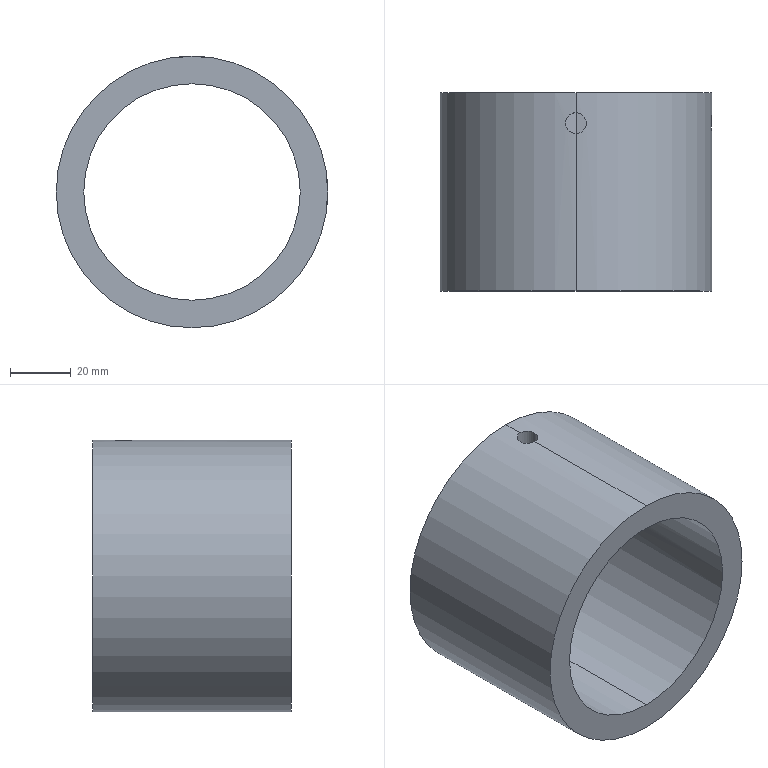Part | SolidWorks | features ICE 2, 3DProfileFeature 1, Extrusion 1, HoleWzd 1 | 1 solid | 10 faces | box 89 x 65 x 89 mm | volume 146372 mm3 | cylinder 8 | plane 2 | commonest cylinder face diameters 6.8 x4 71 x2 89 x2
STEP:
#1=CARTESIAN_POINT('',(0.,51.6,35.5));
#2=VERTEX_POINT('',#1);
#3=CARTESIAN_POINT('',(-3.4,55.,35.337));
#4=VERTEX_POINT('',#3);
#5=CARTESIAN_POINT('',(0.,51.6,35.5));
#6=CARTESIAN_POINT('',(-0.2219,51.6,35.5));
#7=CARTESIAN_POINT('',(-0.4472,51.622,35.498));
#8=CARTESIAN_POINT('',(-0.8832,51.709,35.49));
#9=CARTESIAN_POINT('',(-1.095,51.774,35.484));
#10=CARTESIAN_POINT('',(-1.507,51.944,35.469));
#11=CARTESIAN_POINT('',(-1.706,52.051,35.459));
#12=CARTESIAN_POINT('',(-2.074,52.297,35.44));
#13=CARTESIAN_POINT('',(-2.246,52.437,35.429));
#14=CARTESIAN_POINT('',(-2.563,52.755,35.408));
#15=CARTESIAN_POINT('',(-2.703,52.926,35.397));
#16=CARTESIAN_POINT('',(-2.95,53.294,35.377));
#17=CARTESIAN_POINT('',(-3.056,53.493,35.368));
#18=CARTESIAN_POINT('',(-3.227,53.905,35.353));
#19=CARTESIAN_POINT('',(-3.291,54.117,35.347));
#20=CARTESIAN_POINT('',(-3.378,54.553,35.339));
#21=CARTESIAN_POINT('',(-3.4,54.778,35.337));
#22=CARTESIAN_POINT('',(-3.4,55.,35.337));
#23=B_SPLINE_CURVE_WITH_KNOTS('',3,(#5,#6,#7,#8,#9,#10,#11,#12,#13,#14,#15,#16,#17,#18,#19,#20,#21,#22),.UNSPECIFIED.,.F.,.F.,(4,2,2,2,2,2,2,2,4),(0.005319,0.005984,0.006648,0.007313,0.007978,0.008642,0.009307,0.009971,0.01064),.UNSPECIFIED.);
#24=EDGE_CURVE('',#2,#4,#23,.T.);
#25=ORIENTED_EDGE('',*,*,#24,.T.);
#26=CARTESIAN_POINT('',(-3.4,55.,44.37));
#27=VERTEX_POINT('',#26);
#28=CARTESIAN_POINT('',(-3.4,55.,34.5));
#29=DIRECTION('',(0.,0.,1.));
#30=VECTOR('',#29,1000.);
#31=LINE('',#28,#30);
#32=EDGE_CURVE('',#4,#27,#31,.T.);
#33=ORIENTED_EDGE('',*,*,#32,.T.);
#34=CARTESIAN_POINT('',(0.,51.6,44.5));
#35=VERTEX_POINT('',#34);
#36=CARTESIAN_POINT('',(0.,51.6,44.5));
#37=CARTESIAN_POINT('',(-0.2218,51.6,44.5));
#38=CARTESIAN_POINT('',(-0.4471,51.622,44.498));
#39=CARTESIAN_POINT('',(-0.8831,51.709,44.492));
#40=CARTESIAN_POINT('',(-1.095,51.773,44.487));
#41=CARTESIAN_POINT('',(-1.507,51.944,44.475));
#42=CARTESIAN_POINT('',(-1.706,52.05,44.468));
#43=CARTESIAN_POINT('',(-2.074,52.297,44.452));
#44=CARTESIAN_POINT('',(-2.245,52.437,44.444));
#45=CARTESIAN_POINT('',(-2.563,52.755,44.426));
#46=CARTESIAN_POINT('',(-2.703,52.926,44.418));
#47=CARTESIAN_POINT('',(-2.95,53.294,44.402));
#48=CARTESIAN_POINT('',(-3.056,53.493,44.395));
#49=CARTESIAN_POINT('',(-3.227,53.905,44.383));
#50=CARTESIAN_POINT('',(-3.291,54.117,44.378));
#51=CARTESIAN_POINT('',(-3.378,54.553,44.372));
#52=CARTESIAN_POINT('',(-3.4,54.778,44.37));
#53=CARTESIAN_POINT('',(-3.4,55.,44.37));
#54=B_SPLINE_CURVE_WITH_KNOTS('',3,(#36,#37,#38,#39,#40,#41,#42,#43,#44,#45,#46,#47,#48,#49,#50,#51,#52,#53),.UNSPECIFIED.,.F.,.F.,(4,2,2,2,2,2,2,2,4),(0.005318,0.005983,0.006647,0.007312,0.007976,0.00864,0.009305,0.009969,0.01063),.UNSPECIFIED.);
#55=EDGE_CURVE('',#35,#27,#54,.T.);
#56=ORIENTED_EDGE('',*,*,#55,.F.);
#57=CARTESIAN_POINT('',(3.4,55.,44.37));
#58=VERTEX_POINT('',#57);
#59=CARTESIAN_POINT('',(3.4,55.,44.37));
#60=CARTESIAN_POINT('',(3.4,54.775,44.37));
#61=CARTESIAN_POINT('',(3.378,54.554,44.372));
#62=CARTESIAN_POINT('',(3.291,54.119,44.378));
#63=CARTESIAN_POINT('',(3.226,53.903,44.383));
#64=CARTESIAN_POINT('',(3.055,53.492,44.395));
#65=CARTESIAN_POINT('',(2.951,53.296,44.402));
#66=CARTESIAN_POINT('',(2.704,52.927,44.418));
#67=CARTESIAN_POINT('',(2.56,52.752,44.427));
#68=CARTESIAN_POINT('',(2.246,52.438,44.444));
#69=CARTESIAN_POINT('',(2.075,52.297,44.452));
#70=CARTESIAN_POINT('',(1.703,52.049,44.468));
#71=CARTESIAN_POINT('',(1.505,51.943,44.475));
#72=CARTESIAN_POINT('',(1.096,51.774,44.487));
#73=CARTESIAN_POINT('',(0.8817,51.709,44.492));
#74=CARTESIAN_POINT('',(0.4426,51.622,44.498));
#75=CARTESIAN_POINT('',(0.2219,51.6,44.5));
#76=CARTESIAN_POINT('',(0.,51.6,44.5));
#77=B_SPLINE_CURVE_WITH_KNOTS('',3,(#59,#60,#61,#62,#63,#64,#65,#66,#67,#68,#69,#70,#71,#72,#73,#74,#75,#76),.UNSPECIFIED.,.F.,.F.,(4,2,2,2,2,2,2,2,4),(0.,0.0006648,0.00133,0.001994,0.002659,0.003324,0.003989,0.004653,0.005318),.UNSPECIFIED.);
#78=EDGE_CURVE('',#58,#35,#77,.T.);
#79=ORIENTED_EDGE('',*,*,#78,.F.);
#80=CARTESIAN_POINT('',(3.4,55.,35.337));
#81=VERTEX_POINT('',#80);
#82=CARTESIAN_POINT('',(3.4,55.,34.5));
#83=DIRECTION('',(0.,0.,1.));
#84=VECTOR('',#83,1000.);
#85=LINE('',#82,#84);
#86=EDGE_CURVE('',#81,#58,#85,.T.);
#87=ORIENTED_EDGE('',*,*,#86,.F.);
#88=CARTESIAN_POINT('',(3.4,55.,35.337));
#89=CARTESIAN_POINT('',(3.4,54.775,35.337));
#90=CARTESIAN_POINT('',(3.378,54.554,35.339));
#91=CARTESIAN_POINT('',(3.291,54.119,35.347));
#92=CARTESIAN_POINT('',(3.226,53.903,35.353));
#93=CARTESIAN_POINT('',(3.055,53.491,35.368));
#94=CARTESIAN_POINT('',(2.951,53.296,35.377));
#95=CARTESIAN_POINT('',(2.704,52.927,35.397));
#96=CARTESIAN_POINT('',(2.56,52.752,35.408));
#97=CARTESIAN_POINT('',(2.246,52.438,35.429));
#98=CARTESIAN_POINT('',(2.075,52.298,35.44));
#99=CARTESIAN_POINT('',(1.703,52.049,35.46));
#100=CARTESIAN_POINT('',(1.506,51.943,35.469));
#101=CARTESIAN_POINT('',(1.096,51.774,35.484));
#102=CARTESIAN_POINT('',(0.8818,51.709,35.49));
#103=CARTESIAN_POINT('',(0.4427,51.622,35.498));
#104=CARTESIAN_POINT('',(0.222,51.6,35.5));
#105=CARTESIAN_POINT('',(0.,51.6,35.5));
#106=B_SPLINE_CURVE_WITH_KNOTS('',3,(#88,#89,#90,#91,#92,#93,#94,#95,#96,#97,#98,#99,#100,#101,#102,#103,#104,#105),.UNSPECIFIED.,.F.,.F.,(4,2,2,2,2,2,2,2,4),(0.,0.0006649,0.00133,0.001995,0.00266,0.003325,0.003989,0.004654,0.005319),.UNSPECIFIED.);
#107=EDGE_CURVE('',#81,#2,#106,.T.);
#108=ORIENTED_EDGE('',*,*,#107,.T.);
#109=EDGE_LOOP('',(#25,#33,#56,#79,#87,#108));
#110=FACE_OUTER_BOUND('',#109,.T.);
#111=CARTESIAN_POINT('',(0.,55.,34.5));
#112=DIRECTION('',(0.,0.,1.));
#113=DIRECTION('',(1.,0.,0.));
#114=AXIS2_PLACEMENT_3D('',#111,#112,#113);
#115=CYLINDRICAL_SURFACE('',#114,3.4);
#116=ADVANCED_FACE('',(#110),#115,.F.);
#117=CARTESIAN_POINT('',(35.337,55.,-3.4));
#118=VERTEX_POINT('',#117);
#119=CARTESIAN_POINT('',(35.337,55.,3.4));
#120=VERTEX_POINT('',#119);
#121=CARTESIAN_POINT('',(35.337,55.,-3.4));
#122=CARTESIAN_POINT('',(35.337,54.775,-3.4));
#123=CARTESIAN_POINT('',(35.339,54.554,-3.378));
#124=CARTESIAN_POINT('',(35.347,54.119,-3.291));
#125=CARTESIAN_POINT('',(35.353,53.903,-3.226));
#126=CARTESIAN_POINT('',(35.368,53.492,-3.055));
#127=CARTESIAN_POINT('',(35.377,53.296,-2.951));
#128=CARTESIAN_POINT('',(35.397,52.927,-2.704));
#129=CARTESIAN_POINT('',(35.408,52.752,-2.56));
#130=CARTESIAN_POINT('',(35.429,52.439,-2.247));
#131=CARTESIAN_POINT('',(35.44,52.298,-2.076));
#132=CARTESIAN_POINT('',(35.46,52.049,-1.704));
#133=CARTESIAN_POINT('',(35.469,51.944,-1.506));
#134=CARTESIAN_POINT('',(35.484,51.774,-1.097));
#135=CARTESIAN_POINT('',(35.49,51.709,-0.8828));
#136=CARTESIAN_POINT('',(35.498,51.622,-0.4438));
#137=CARTESIAN_POINT('',(35.5,51.6,-0.2231));
#138=CARTESIAN_POINT('',(35.5,51.6,0.2207));
#139=CARTESIAN_POINT('',(35.498,51.622,0.4461));
#140=CARTESIAN_POINT('',(35.49,51.709,0.8823));
#141=CARTESIAN_POINT('',(35.484,51.773,1.094));
#142=CARTESIAN_POINT('',(35.469,51.944,1.506));
#143=CARTESIAN_POINT('',(35.46,52.05,1.705));
#144=CARTESIAN_POINT('',(35.44,52.296,2.073));
#145=CARTESIAN_POINT('',(35.429,52.437,2.245));
#146=CARTESIAN_POINT('',(35.408,52.754,2.563));
#147=CARTESIAN_POINT('',(35.397,52.926,2.703));
#148=CARTESIAN_POINT('',(35.377,53.294,2.949));
#149=CARTESIAN_POINT('',(35.368,53.493,3.056));
#150=CARTESIAN_POINT('',(35.353,53.905,3.226));
#151=CARTESIAN_POINT('',(35.347,54.117,3.291));
#152=CARTESIAN_POINT('',(35.339,54.553,3.378));
#153=CARTESIAN_POINT('',(35.337,54.778,3.4));
#154=CARTESIAN_POINT('',(35.337,55.,3.4));
#155=B_SPLINE_CURVE_WITH_KNOTS('',3,(#121,#122,#123,#124,#125,#126,#127,#128,#129,#130,#131,#132,#133,#134,#135,#136,#137,#138,#139,#140,#141,#142,#143,#144,#145,#146,#147,#148,#149,#150,#151,#152,#153,#154),.UNSPECIFIED.,.F.,.F.,(4,2,2,2,2,2,2,2,2,2,2,2,2,2,2,2,4),(0.,0.0006648,0.00133,0.001994,0.002659,0.003324,0.003989,0.004653,0.005318,0.005983,0.006648,0.007312,0.007977,0.008642,0.009307,0.009971,0.01064),.UNSPECIFIED.);
#156=EDGE_CURVE('',#118,#120,#155,.T.);
#157=ORIENTED_EDGE('',*,*,#156,.T.);
#158=CARTESIAN_POINT('',(44.37,55.,3.4));
#159=VERTEX_POINT('',#158);
#160=CARTESIAN_POINT('',(34.5,55.,3.4));
#161=DIRECTION('',(1.,0.,0.));
#162=VECTOR('',#161,1000.);
#163=LINE('',#160,#162);
#164=EDGE_CURVE('',#120,#159,#163,.T.);
#165=ORIENTED_EDGE('',*,*,#164,.T.);
#166=CARTESIAN_POINT('',(44.37,55.,-3.4));
#167=VERTEX_POINT('',#166);
#168=CARTESIAN_POINT('',(44.37,55.,-3.4));
#169=CARTESIAN_POINT('',(44.37,54.775,-3.4));
#170=CARTESIAN_POINT('',(44.372,54.554,-3.378));
#171=CARTESIAN_POINT('',(44.378,54.12,-3.292));
#172=CARTESIAN_POINT('',(44.383,53.904,-3.226));
#173=CARTESIAN_POINT('',(44.395,53.492,-3.055));
#174=CARTESIAN_POINT('',(44.402,53.297,-2.951));
#175=CARTESIAN_POINT('',(44.418,52.927,-2.704));
#176=CARTESIAN_POINT('',(44.427,52.752,-2.561));
#177=CARTESIAN_POINT('',(44.444,52.439,-2.247));
#178=CARTESIAN_POINT('',(44.452,52.298,-2.076));
#179=CARTESIAN_POINT('',(44.468,52.049,-1.704));
#180=CARTESIAN_POINT('',(44.475,51.944,-1.506));
#181=CARTESIAN_POINT('',(44.487,51.774,-1.097));
#182=CARTESIAN_POINT('',(44.492,51.709,-0.8827));
#183=CARTESIAN_POINT('',(44.498,51.622,-0.4438));
#184=CARTESIAN_POINT('',(44.5,51.6,-0.2231));
#185=CARTESIAN_POINT('',(44.5,51.6,0.2206));
#186=CARTESIAN_POINT('',(44.498,51.622,0.446));
#187=CARTESIAN_POINT('',(44.492,51.709,0.8821));
#188=CARTESIAN_POINT('',(44.487,51.773,1.094));
#189=CARTESIAN_POINT('',(44.475,51.944,1.506));
#190=CARTESIAN_POINT('',(44.468,52.05,1.705));
#191=CARTESIAN_POINT('',(44.452,52.296,2.073));
#192=CARTESIAN_POINT('',(44.444,52.437,2.245));
#193=CARTESIAN_POINT('',(44.426,52.754,2.562));
#194=CARTESIAN_POINT('',(44.418,52.926,2.703));
#195=CARTESIAN_POINT('',(44.402,53.294,2.949));
#196=CARTESIAN_POINT('',(44.395,53.493,3.056));
#197=CARTESIAN_POINT('',(44.383,53.905,3.226));
#198=CARTESIAN_POINT('',(44.378,54.117,3.291));
#199=CARTESIAN_POINT('',(44.372,54.553,3.378));
#200=CARTESIAN_POINT('',(44.37,54.778,3.4));
#201=CARTESIAN_POINT('',(44.37,55.,3.4));
#202=B_SPLINE_CURVE_WITH_KNOTS('',3,(#168,#169,#170,#171,#172,#173,#174,#175,#176,#177,#178,#179,#180,#181,#182,#183,#184,#185,#186,#187,#188,#189,#190,#191,#192,#193,#194,#195,#196,#197,#198,#199,#200,#201),.UNSPECIFIED.,.F.,.F.,(4,2,2,2,2,2,2,2,2,2,2,2,2,2,2,2,4),(0.,0.0006646,0.001329,0.001994,0.002658,0.003323,0.003988,0.004652,0.005317,0.005982,0.006646,0.007311,0.007975,0.00864,0.009305,0.009969,0.01063),.UNSPECIFIED.);
#203=EDGE_CURVE('',#167,#159,#202,.T.);
#204=ORIENTED_EDGE('',*,*,#203,.F.);
#205=CARTESIAN_POINT('',(34.5,55.,-3.4));
#206=DIRECTION('',(1.,0.,0.));
#207=VECTOR('',#206,1000.);
#208=LINE('',#205,#207);
#209=EDGE_CURVE('',#118,#167,#208,.T.);
#210=ORIENTED_EDGE('',*,*,#209,.F.);
#211=EDGE_LOOP('',(#157,#165,#204,#210));
#212=FACE_OUTER_BOUND('',#211,.T.);
#213=CARTESIAN_POINT('',(34.5,55.,0.));
#214=DIRECTION('',(1.,0.,0.));
#215=DIRECTION('',(0.,0.,-1.));
#216=AXIS2_PLACEMENT_3D('',#213,#214,#215);
#217=CYLINDRICAL_SURFACE('',#216,3.4);
#218=ADVANCED_FACE('',(#212),#217,.F.);
#219=CARTESIAN_POINT('',(0.,65.,-35.5));
#220=VERTEX_POINT('',#219);
#221=CARTESIAN_POINT('',(0.,65.,35.5));
#222=VERTEX_POINT('',#221);
#223=CARTESIAN_POINT('',(0.,65.,0.));
#224=DIRECTION('',(0.,1.,0.));
#225=DIRECTION('',(0.,0.,1.));
#226=AXIS2_PLACEMENT_3D('',#223,#224,#225);
#227=CIRCLE('',#226,35.5);
#228=EDGE_CURVE('',#220,#222,#227,.T.);
#229=ORIENTED_EDGE('',*,*,#228,.T.);
#230=CARTESIAN_POINT('',(0.,58.4,35.5));
#231=VERTEX_POINT('',#230);
#232=CARTESIAN_POINT('',(0.,65.,35.5));
#233=DIRECTION('',(0.,-1.,0.));
#234=VECTOR('',#233,1000.);
#235=LINE('',#232,#234);
#236=EDGE_CURVE('',#222,#231,#235,.T.);
#237=ORIENTED_EDGE('',*,*,#236,.T.);
#238=CARTESIAN_POINT('',(-3.4,55.,35.337));
#239=CARTESIAN_POINT('',(-3.4,55.222,35.337));
#240=CARTESIAN_POINT('',(-3.378,55.443,35.339));
#241=CARTESIAN_POINT('',(-3.291,55.882,35.347));
#242=CARTESIAN_POINT('',(-3.226,56.096,35.353));
#243=CARTESIAN_POINT('',(-3.056,56.506,35.368));
#244=CARTESIAN_POINT('',(-2.951,56.703,35.377));
#245=CARTESIAN_POINT('',(-2.702,57.075,35.397));
#246=CARTESIAN_POINT('',(-2.562,57.247,35.408));
#247=CARTESIAN_POINT('',(-2.248,57.56,35.429));
#248=CARTESIAN_POINT('',(-2.073,57.704,35.44));
#249=CARTESIAN_POINT('',(-1.704,57.951,35.46));
#250=CARTESIAN_POINT('',(-1.508,58.055,35.469));
#251=CARTESIAN_POINT('',(-1.097,58.226,35.484));
#252=CARTESIAN_POINT('',(-0.8806,58.291,35.49));
#253=CARTESIAN_POINT('',(-0.4457,58.378,35.498));
#254=CARTESIAN_POINT('',(-0.2247,58.4,35.5));
#255=CARTESIAN_POINT('',(0.,58.4,35.5));
#256=B_SPLINE_CURVE_WITH_KNOTS('',3,(#238,#239,#240,#241,#242,#243,#244,#245,#246,#247,#248,#249,#250,#251,#252,#253,#254,#255),.UNSPECIFIED.,.F.,.F.,(4,2,2,2,2,2,2,2,4),(0.01064,0.0113,0.01197,0.01263,0.0133,0.01396,0.01463,0.01529,0.01596),.UNSPECIFIED.);
#257=EDGE_CURVE('',#4,#231,#256,.T.);
#258=ORIENTED_EDGE('',*,*,#257,.F.);
#259=ORIENTED_EDGE('',*,*,#24,.F.);
#260=CARTESIAN_POINT('',(0.,0.,35.5));
#261=VERTEX_POINT('',#260);
#262=CARTESIAN_POINT('',(0.,65.,35.5));
#263=DIRECTION('',(0.,-1.,0.));
#264=VECTOR('',#263,1000.);
#265=LINE('',#262,#264);
#266=EDGE_CURVE('',#2,#261,#265,.T.);
#267=ORIENTED_EDGE('',*,*,#266,.T.);
#268=CARTESIAN_POINT('',(0.,0.,-35.5));
#269=VERTEX_POINT('',#268);
#270=CARTESIAN_POINT('',(0.,0.,0.));
#271=DIRECTION('',(0.,1.,0.));
#272=DIRECTION('',(0.,0.,1.));
#273=AXIS2_PLACEMENT_3D('',#270,#271,#272);
#274=CIRCLE('',#273,35.5);
#275=EDGE_CURVE('',#269,#261,#274,.T.);
#276=ORIENTED_EDGE('',*,*,#275,.F.);
#277=CARTESIAN_POINT('',(0.,65.,-35.5));
#278=DIRECTION('',(0.,-1.,0.));
#279=VECTOR('',#278,1000.);
#280=LINE('',#277,#279);
#281=EDGE_CURVE('',#220,#269,#280,.T.);
#282=ORIENTED_EDGE('',*,*,#281,.F.);
#283=EDGE_LOOP('',(#229,#237,#258,#259,#267,#276,#282));
#284=FACE_OUTER_BOUND('',#283,.T.);
#285=CARTESIAN_POINT('',(0.,65.,0.));
#286=DIRECTION('',(0.,-1.,0.));
#287=DIRECTION('',(0.,0.,-1.));
#288=AXIS2_PLACEMENT_3D('',#285,#286,#287);
#289=CYLINDRICAL_SURFACE('',#288,35.5);
#290=ADVANCED_FACE('',(#284),#289,.F.);
#291=ORIENTED_EDGE('',*,*,#203,.T.);
#292=CARTESIAN_POINT('',(44.37,55.,3.4));
#293=CARTESIAN_POINT('',(44.37,55.222,3.4));
#294=CARTESIAN_POINT('',(44.372,55.442,3.378));
#295=CARTESIAN_POINT('',(44.378,55.881,3.291));
#296=CARTESIAN_POINT('',(44.383,56.096,3.226));
#297=CARTESIAN_POINT('',(44.395,56.505,3.057));
#298=CARTESIAN_POINT('',(44.402,56.702,2.952));
#299=CARTESIAN_POINT('',(44.418,57.074,2.703));
#300=CARTESIAN_POINT('',(44.426,57.246,2.562));
#301=CARTESIAN_POINT('',(44.443,57.559,2.249));
#302=CARTESIAN_POINT('',(44.452,57.703,2.075));
#303=CARTESIAN_POINT('',(44.468,57.95,1.705));
#304=CARTESIAN_POINT('',(44.475,58.054,1.51));
#305=CARTESIAN_POINT('',(44.487,58.225,1.099));
#306=CARTESIAN_POINT('',(44.492,58.291,0.8825));
#307=CARTESIAN_POINT('',(44.498,58.378,0.4479));
#308=CARTESIAN_POINT('',(44.5,58.4,0.2271));
#309=CARTESIAN_POINT('',(44.5,58.4,-0.2217));
#310=CARTESIAN_POINT('',(44.498,58.378,-0.4432));
#311=CARTESIAN_POINT('',(44.492,58.292,-0.8778));
#312=CARTESIAN_POINT('',(44.487,58.227,-1.094));
#313=CARTESIAN_POINT('',(44.475,58.057,-1.506));
#314=CARTESIAN_POINT('',(44.468,57.952,-1.701));
#315=CARTESIAN_POINT('',(44.452,57.706,-2.07));
#316=CARTESIAN_POINT('',(44.444,57.563,-2.246));
#317=CARTESIAN_POINT('',(44.427,57.249,-2.559));
#318=CARTESIAN_POINT('',(44.418,57.078,-2.7));
#319=CARTESIAN_POINT('',(44.402,56.707,-2.949));
#320=CARTESIAN_POINT('',(44.395,56.509,-3.055));
#321=CARTESIAN_POINT('',(44.383,56.1,-3.225));
#322=CARTESIAN_POINT('',(44.378,55.887,-3.29));
#323=CARTESIAN_POINT('',(44.372,55.447,-3.378));
#324=CARTESIAN_POINT('',(44.37,55.225,-3.4));
#325=CARTESIAN_POINT('',(44.37,55.,-3.4));
#326=B_SPLINE_CURVE_WITH_KNOTS('',3,(#292,#293,#294,#295,#296,#297,#298,#299,#300,#301,#302,#303,#304,#305,#306,#307,#308,#309,#310,#311,#312,#313,#314,#315,#316,#317,#318,#319,#320,#321,#322,#323,#324,#325),.UNSPECIFIED.,.F.,.F.,(4,2,2,2,2,2,2,2,2,2,2,2,2,2,2,2,4),(0.01063,0.0113,0.01196,0.01263,0.01329,0.01396,0.01462,0.01529,0.01595,0.01661,0.01728,0.01794,0.01861,0.01927,0.01994,0.0206,0.02127),.UNSPECIFIED.);
#327=EDGE_CURVE('',#159,#167,#326,.T.);
#328=ORIENTED_EDGE('',*,*,#327,.T.);
#329=EDGE_LOOP('',(#291,#328));
#330=FACE_BOUND('',#329,.T.);
#331=CARTESIAN_POINT('',(0.,65.,44.5));
#332=VERTEX_POINT('',#331);
#333=CARTESIAN_POINT('',(0.,65.,-44.5));
#334=VERTEX_POINT('',#333);
#335=CARTESIAN_POINT('',(0.,65.,0.));
#336=DIRECTION('',(0.,1.,0.));
#337=DIRECTION('',(0.,0.,1.));
#338=AXIS2_PLACEMENT_3D('',#335,#336,#337);
#339=CIRCLE('',#338,44.5);
#340=EDGE_CURVE('',#332,#334,#339,.T.);
#341=ORIENTED_EDGE('',*,*,#340,.F.);
#342=CARTESIAN_POINT('',(0.,58.4,44.5));
#343=VERTEX_POINT('',#342);
#344=CARTESIAN_POINT('',(0.,65.,44.5));
#345=DIRECTION('',(0.,-1.,0.));
#346=VECTOR('',#345,1000.);
#347=LINE('',#344,#346);
#348=EDGE_CURVE('',#332,#343,#347,.T.);
#349=ORIENTED_EDGE('',*,*,#348,.T.);
#350=CARTESIAN_POINT('',(0.,58.4,44.5));
#351=CARTESIAN_POINT('',(0.2243,58.4,44.5));
#352=CARTESIAN_POINT('',(0.4457,58.378,44.498));
#353=CARTESIAN_POINT('',(0.88,58.292,44.492));
#354=CARTESIAN_POINT('',(1.096,58.226,44.487));
#355=CARTESIAN_POINT('',(1.507,58.056,44.475));
#356=CARTESIAN_POINT('',(1.703,57.951,44.468));
#357=CARTESIAN_POINT('',(2.072,57.705,44.452));
#358=CARTESIAN_POINT('',(2.247,57.562,44.444));
#359=CARTESIAN_POINT('',(2.56,57.248,44.427));
#360=CARTESIAN_POINT('',(2.701,57.077,44.418));
#361=CARTESIAN_POINT('',(2.949,56.706,44.402));
#362=CARTESIAN_POINT('',(3.055,56.508,44.395));
#363=CARTESIAN_POINT('',(3.225,56.1,44.383));
#364=CARTESIAN_POINT('',(3.29,55.886,44.378));
#365=CARTESIAN_POINT('',(3.378,55.447,44.372));
#366=CARTESIAN_POINT('',(3.4,55.225,44.37));
#367=CARTESIAN_POINT('',(3.4,55.,44.37));
#368=B_SPLINE_CURVE_WITH_KNOTS('',3,(#350,#351,#352,#353,#354,#355,#356,#357,#358,#359,#360,#361,#362,#363,#364,#365,#366,#367),.UNSPECIFIED.,.F.,.F.,(4,2,2,2,2,2,2,2,4),(0.01595,0.01662,0.01728,0.01794,0.01861,0.01927,0.01994,0.0206,0.02127),.UNSPECIFIED.);
#369=EDGE_CURVE('',#343,#58,#368,.T.);
#370=ORIENTED_EDGE('',*,*,#369,.T.);
#371=ORIENTED_EDGE('',*,*,#78,.T.);
#372=CARTESIAN_POINT('',(0.,0.,44.5));
#373=VERTEX_POINT('',#372);
#374=CARTESIAN_POINT('',(0.,65.,44.5));
#375=DIRECTION('',(0.,-1.,0.));
#376=VECTOR('',#375,1000.);
#377=LINE('',#374,#376);
#378=EDGE_CURVE('',#35,#373,#377,.T.);
#379=ORIENTED_EDGE('',*,*,#378,.T.);
#380=CARTESIAN_POINT('',(0.,0.,-44.5));
#381=VERTEX_POINT('',#380);
#382=CARTESIAN_POINT('',(0.,0.,0.));
#383=DIRECTION('',(0.,1.,0.));
#384=DIRECTION('',(0.,0.,1.));
#385=AXIS2_PLACEMENT_3D('',#382,#383,#384);
#386=CIRCLE('',#385,44.5);
#387=EDGE_CURVE('',#373,#381,#386,.T.);
#388=ORIENTED_EDGE('',*,*,#387,.T.);
#389=CARTESIAN_POINT('',(0.,65.,-44.5));
#390=DIRECTION('',(0.,-1.,0.));
#391=VECTOR('',#390,1000.);
#392=LINE('',#389,#391);
#393=EDGE_CURVE('',#334,#381,#392,.T.);
#394=ORIENTED_EDGE('',*,*,#393,.F.);
#395=EDGE_LOOP('',(#341,#349,#370,#371,#379,#388,#394));
#396=FACE_OUTER_BOUND('',#395,.T.);
#397=CARTESIAN_POINT('',(0.,65.,0.));
#398=DIRECTION('',(0.,-1.,0.));
#399=DIRECTION('',(0.,0.,-1.));
#400=AXIS2_PLACEMENT_3D('',#397,#398,#399);
#401=CYLINDRICAL_SURFACE('',#400,44.5);
#402=ADVANCED_FACE('',(#330,#396),#401,.T.);
#403=CARTESIAN_POINT('',(0.,65.,0.));
#404=DIRECTION('',(0.,1.,0.));
#405=DIRECTION('',(0.,0.,1.));
#406=AXIS2_PLACEMENT_3D('',#403,#404,#405);
#407=CIRCLE('',#406,44.5);
#408=EDGE_CURVE('',#334,#332,#407,.T.);
#409=ORIENTED_EDGE('',*,*,#408,.T.);
#410=ORIENTED_EDGE('',*,*,#340,.T.);
#411=EDGE_LOOP('',(#409,#410));
#412=FACE_OUTER_BOUND('',#411,.T.);
#413=ORIENTED_EDGE('',*,*,#228,.F.);
#414=CARTESIAN_POINT('',(0.,65.,0.));
#415=DIRECTION('',(0.,1.,0.));
#416=DIRECTION('',(0.,0.,1.));
#417=AXIS2_PLACEMENT_3D('',#414,#415,#416);
#418=CIRCLE('',#417,35.5);
#419=EDGE_CURVE('',#222,#220,#418,.T.);
#420=ORIENTED_EDGE('',*,*,#419,.F.);
#421=EDGE_LOOP('',(#413,#420));
#422=FACE_BOUND('',#421,.T.);
#423=CARTESIAN_POINT('',(0.,65.,0.));
#424=DIRECTION('',(0.,1.,0.));
#425=DIRECTION('',(0.,0.,1.));
#426=AXIS2_PLACEMENT_3D('',#423,#424,#425);
#427=PLANE('',#426);
#428=ADVANCED_FACE('',(#412,#422),#427,.T.);
#429=CARTESIAN_POINT('',(0.,0.,0.));
#430=DIRECTION('',(0.,1.,0.));
#431=DIRECTION('',(0.,0.,1.));
#432=AXIS2_PLACEMENT_3D('',#429,#430,#431);
#433=CIRCLE('',#432,44.5);
#434=EDGE_CURVE('',#381,#373,#433,.T.);
#435=ORIENTED_EDGE('',*,*,#434,.F.);
#436=ORIENTED_EDGE('',*,*,#387,.F.);
#437=EDGE_LOOP('',(#435,#436));
#438=FACE_OUTER_BOUND('',#437,.T.);
#439=ORIENTED_EDGE('',*,*,#275,.T.);
#440=CARTESIAN_POINT('',(0.,0.,0.));
#441=DIRECTION('',(0.,1.,0.));
#442=DIRECTION('',(0.,0.,1.));
#443=AXIS2_PLACEMENT_3D('',#440,#441,#442);
#444=CIRCLE('',#443,35.5);
#445=EDGE_CURVE('',#261,#269,#444,.T.);
#446=ORIENTED_EDGE('',*,*,#445,.T.);
#447=EDGE_LOOP('',(#439,#446));
#448=FACE_BOUND('',#447,.T.);
#449=CARTESIAN_POINT('',(0.,0.,0.));
#450=DIRECTION('',(0.,1.,0.));
#451=DIRECTION('',(0.,0.,1.));
#452=AXIS2_PLACEMENT_3D('',#449,#450,#451);
#453=PLANE('',#452);
#454=ADVANCED_FACE('',(#438,#448),#453,.F.);
#455=ORIENTED_EDGE('',*,*,#348,.F.);
#456=ORIENTED_EDGE('',*,*,#408,.F.);
#457=ORIENTED_EDGE('',*,*,#393,.T.);
#458=ORIENTED_EDGE('',*,*,#434,.T.);
#459=ORIENTED_EDGE('',*,*,#378,.F.);
#460=ORIENTED_EDGE('',*,*,#55,.T.);
#461=CARTESIAN_POINT('',(-3.4,55.,44.37));
#462=CARTESIAN_POINT('',(-3.4,55.222,44.37));
#463=CARTESIAN_POINT('',(-3.378,55.443,44.372));
#464=CARTESIAN_POINT('',(-3.291,55.881,44.378));
#465=CARTESIAN_POINT('',(-3.226,56.096,44.383));
#466=CARTESIAN_POINT('',(-3.056,56.506,44.395));
#467=CARTESIAN_POINT('',(-2.951,56.703,44.402));
#468=CARTESIAN_POINT('',(-2.702,57.075,44.418));
#469=CARTESIAN_POINT('',(-2.562,57.247,44.426));
#470=CARTESIAN_POINT('',(-2.248,57.56,44.443));
#471=CARTESIAN_POINT('',(-2.073,57.704,44.452));
#472=CARTESIAN_POINT('',(-1.703,57.951,44.468));
#473=CARTESIAN_POINT('',(-1.508,58.055,44.475));
#474=CARTESIAN_POINT('',(-1.097,58.226,44.487));
#475=CARTESIAN_POINT('',(-0.8804,58.292,44.492));
#476=CARTESIAN_POINT('',(-0.4455,58.378,44.498));
#477=CARTESIAN_POINT('',(-0.2246,58.4,44.5));
#478=CARTESIAN_POINT('',(0.,58.4,44.5));
#479=B_SPLINE_CURVE_WITH_KNOTS('',3,(#461,#462,#463,#464,#465,#466,#467,#468,#469,#470,#471,#472,#473,#474,#475,#476,#477,#478),.UNSPECIFIED.,.F.,.F.,(4,2,2,2,2,2,2,2,4),(0.01063,0.0113,0.01196,0.01263,0.01329,0.01396,0.01462,0.01529,0.01595),.UNSPECIFIED.);
#480=EDGE_CURVE('',#27,#343,#479,.T.);
#481=ORIENTED_EDGE('',*,*,#480,.T.);
#482=EDGE_LOOP('',(#455,#456,#457,#458,#459,#460,#481));
#483=FACE_OUTER_BOUND('',#482,.T.);
#484=CARTESIAN_POINT('',(0.,65.,0.));
#485=DIRECTION('',(0.,-1.,0.));
#486=DIRECTION('',(0.,0.,-1.));
#487=AXIS2_PLACEMENT_3D('',#484,#485,#486);
#488=CYLINDRICAL_SURFACE('',#487,44.5);
#489=ADVANCED_FACE('',(#483),#488,.T.);
#490=ORIENTED_EDGE('',*,*,#236,.F.);
#491=ORIENTED_EDGE('',*,*,#419,.T.);
#492=ORIENTED_EDGE('',*,*,#281,.T.);
#493=ORIENTED_EDGE('',*,*,#445,.F.);
#494=ORIENTED_EDGE('',*,*,#266,.F.);
#495=ORIENTED_EDGE('',*,*,#107,.F.);
#496=CARTESIAN_POINT('',(0.,58.4,35.5));
#497=CARTESIAN_POINT('',(0.2245,58.4,35.5));
#498=CARTESIAN_POINT('',(0.4457,58.378,35.498));
#499=CARTESIAN_POINT('',(0.8801,58.292,35.49));
#500=CARTESIAN_POINT('',(1.096,58.226,35.484));
#501=CARTESIAN_POINT('',(1.507,58.056,35.469));
#502=CARTESIAN_POINT('',(1.703,57.951,35.46));
#503=CARTESIAN_POINT('',(2.072,57.705,35.44));
#504=CARTESIAN_POINT('',(2.247,57.562,35.429));
#505=CARTESIAN_POINT('',(2.56,57.248,35.408));
#506=CARTESIAN_POINT('',(2.701,57.077,35.397));
#507=CARTESIAN_POINT('',(2.949,56.706,35.377));
#508=CARTESIAN_POINT('',(3.055,56.509,35.368));
#509=CARTESIAN_POINT('',(3.225,56.1,35.353));
#510=CARTESIAN_POINT('',(3.29,55.886,35.347));
#511=CARTESIAN_POINT('',(3.378,55.447,35.339));
#512=CARTESIAN_POINT('',(3.4,55.225,35.337));
#513=CARTESIAN_POINT('',(3.4,55.,35.337));
#514=B_SPLINE_CURVE_WITH_KNOTS('',3,(#496,#497,#498,#499,#500,#501,#502,#503,#504,#505,#506,#507,#508,#509,#510,#511,#512,#513),.UNSPECIFIED.,.F.,.F.,(4,2,2,2,2,2,2,2,4),(0.01596,0.01662,0.01728,0.01795,0.01861,0.01928,0.01994,0.02061,0.02127),.UNSPECIFIED.);
#515=EDGE_CURVE('',#231,#81,#514,.T.);
#516=ORIENTED_EDGE('',*,*,#515,.F.);
#517=EDGE_LOOP('',(#490,#491,#492,#493,#494,#495,#516));
#518=FACE_OUTER_BOUND('',#517,.T.);
#519=ORIENTED_EDGE('',*,*,#156,.F.);
#520=CARTESIAN_POINT('',(35.337,55.,3.4));
#521=CARTESIAN_POINT('',(35.337,55.222,3.4));
#522=CARTESIAN_POINT('',(35.339,55.443,3.378));
#523=CARTESIAN_POINT('',(35.347,55.881,3.291));
#524=CARTESIAN_POINT('',(35.353,56.096,3.226));
#525=CARTESIAN_POINT('',(35.368,56.505,3.057));
#526=CARTESIAN_POINT('',(35.377,56.703,2.951));
#527=CARTESIAN_POINT('',(35.397,57.075,2.703));
#528=CARTESIAN_POINT('',(35.408,57.246,2.562));
#529=CARTESIAN_POINT('',(35.429,57.559,2.249));
#530=CARTESIAN_POINT('',(35.44,57.703,2.074));
#531=CARTESIAN_POINT('',(35.46,57.95,1.705));
#532=CARTESIAN_POINT('',(35.468,58.054,1.51));
#533=CARTESIAN_POINT('',(35.484,58.225,1.099));
#534=CARTESIAN_POINT('',(35.49,58.291,0.8827));
#535=CARTESIAN_POINT('',(35.498,58.378,0.4481));
#536=CARTESIAN_POINT('',(35.5,58.4,0.2272));
#537=CARTESIAN_POINT('',(35.5,58.4,-0.2219));
#538=CARTESIAN_POINT('',(35.498,58.378,-0.4433));
#539=CARTESIAN_POINT('',(35.49,58.292,-0.878));
#540=CARTESIAN_POINT('',(35.484,58.227,-1.094));
#541=CARTESIAN_POINT('',(35.469,58.057,-1.506));
#542=CARTESIAN_POINT('',(35.46,57.952,-1.701));
#543=CARTESIAN_POINT('',(35.44,57.706,-2.071));
#544=CARTESIAN_POINT('',(35.429,57.562,-2.246));
#545=CARTESIAN_POINT('',(35.408,57.249,-2.559));
#546=CARTESIAN_POINT('',(35.397,57.078,-2.7));
#547=CARTESIAN_POINT('',(35.378,56.707,-2.949));
#548=CARTESIAN_POINT('',(35.368,56.509,-3.055));
#549=CARTESIAN_POINT('',(35.353,56.1,-3.225));
#550=CARTESIAN_POINT('',(35.347,55.887,-3.29));
#551=CARTESIAN_POINT('',(35.339,55.447,-3.378));
#552=CARTESIAN_POINT('',(35.337,55.225,-3.4));
#553=CARTESIAN_POINT('',(35.337,55.,-3.4));
#554=B_SPLINE_CURVE_WITH_KNOTS('',3,(#520,#521,#522,#523,#524,#525,#526,#527,#528,#529,#530,#531,#532,#533,#534,#535,#536,#537,#538,#539,#540,#541,#542,#543,#544,#545,#546,#547,#548,#549,#550,#551,#552,#553),.UNSPECIFIED.,.F.,.F.,(4,2,2,2,2,2,2,2,2,2,2,2,2,2,2,2,4),(0.01064,0.0113,0.01197,0.01263,0.01329,0.01396,0.01462,0.01529,0.01595,0.01662,0.01728,0.01795,0.01861,0.01928,0.01994,0.0206,0.02127),.UNSPECIFIED.);
#555=EDGE_CURVE('',#120,#118,#554,.T.);
#556=ORIENTED_EDGE('',*,*,#555,.F.);
#557=EDGE_LOOP('',(#519,#556));
#558=FACE_BOUND('',#557,.T.);
#559=CARTESIAN_POINT('',(0.,65.,0.));
#560=DIRECTION('',(0.,-1.,0.));
#561=DIRECTION('',(0.,0.,-1.));
#562=AXIS2_PLACEMENT_3D('',#559,#560,#561);
#563=CYLINDRICAL_SURFACE('',#562,35.5);
#564=ADVANCED_FACE('',(#518,#558),#563,.F.);
#565=ORIENTED_EDGE('',*,*,#164,.F.);
#566=ORIENTED_EDGE('',*,*,#555,.T.);
#567=ORIENTED_EDGE('',*,*,#209,.T.);
#568=ORIENTED_EDGE('',*,*,#327,.F.);
#569=EDGE_LOOP('',(#565,#566,#567,#568));
#570=FACE_OUTER_BOUND('',#569,.T.);
#571=CARTESIAN_POINT('',(34.5,55.,0.));
#572=DIRECTION('',(1.,0.,0.));
#573=DIRECTION('',(0.,0.,-1.));
#574=AXIS2_PLACEMENT_3D('',#571,#572,#573);
#575=CYLINDRICAL_SURFACE('',#574,3.4);
#576=ADVANCED_FACE('',(#570),#575,.F.);
#577=ORIENTED_EDGE('',*,*,#32,.F.);
#578=ORIENTED_EDGE('',*,*,#257,.T.);
#579=ORIENTED_EDGE('',*,*,#515,.T.);
#580=ORIENTED_EDGE('',*,*,#86,.T.);
#581=ORIENTED_EDGE('',*,*,#369,.F.);
#582=ORIENTED_EDGE('',*,*,#480,.F.);
#583=EDGE_LOOP('',(#577,#578,#579,#580,#581,#582));
#584=FACE_OUTER_BOUND('',#583,.T.);
#585=CARTESIAN_POINT('',(0.,55.,34.5));
#586=DIRECTION('',(0.,0.,1.));
#587=DIRECTION('',(1.,0.,0.));
#588=AXIS2_PLACEMENT_3D('',#585,#586,#587);
#589=CYLINDRICAL_SURFACE('',#588,3.4);
#590=ADVANCED_FACE('',(#584),#589,.F.);
#591=CLOSED_SHELL('',(#116,#218,#290,#402,#428,#454,#489,#564,#576,#590));
#592=MANIFOLD_SOLID_BREP('',#591);
#593=CARTESIAN_POINT('',(0.,0.,0.));
#594=DIRECTION('',(0.,0.,1.));
#595=DIRECTION('',(1.,0.,0.));
#596=AXIS2_PLACEMENT_3D('',#593,#594,#595);
#597=(LENGTH_UNIT()NAMED_UNIT(*)SI_UNIT(.MILLI.,.METRE.));
#598=UNCERTAINTY_MEASURE_WITH_UNIT(LENGTH_MEASURE(0.00001),#597,'','');
#599=(NAMED_UNIT(*)PLANE_ANGLE_UNIT()SI_UNIT($,.RADIAN.));
#600=(NAMED_UNIT(*)SI_UNIT($,.STERADIAN.)SOLID_ANGLE_UNIT());
#601=(GEOMETRIC_REPRESENTATION_CONTEXT(3)GLOBAL_UNCERTAINTY_ASSIGNED_CONTEXT((#598))GLOBAL_UNIT_ASSIGNED_CONTEXT((#597,#599,#600))REPRESENTATION_CONTEXT('',''));
#602=ADVANCED_BREP_SHAPE_REPRESENTATION('',(#592,#596),#601);